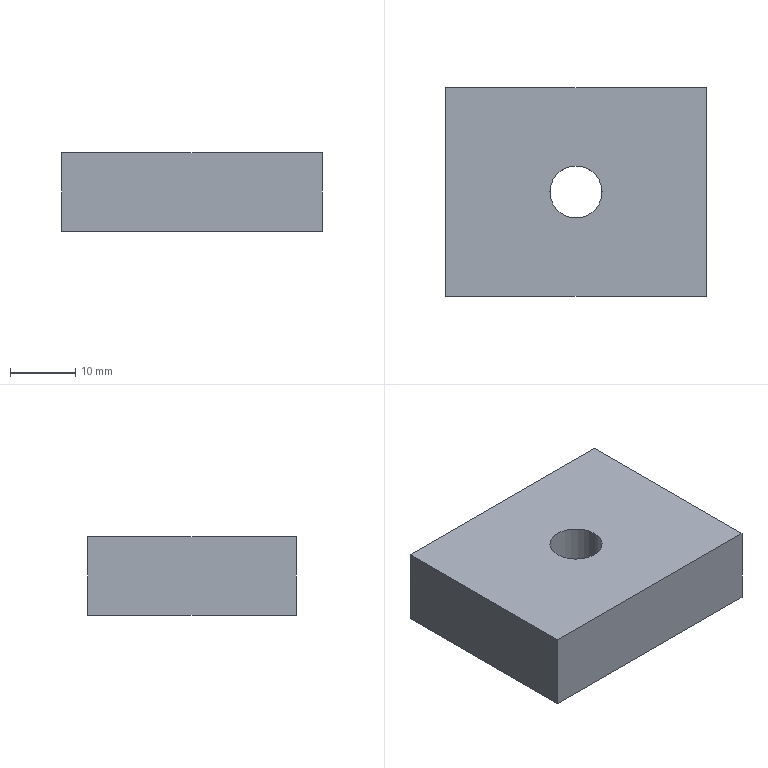Part | STEP file | [02]-4 | 1 solid | 8 faces | box 40 x 32 x 12 mm | volume 14757 mm3 | plane 6 | cylinder 2 | commonest cylinder face diameters 8 x2
STEP:
#1=CARTESIAN_POINT('',(16.,16.,0.));
#2=VERTEX_POINT('',#1);
#3=CARTESIAN_POINT('',(24.,16.,0.));
#4=VERTEX_POINT('',#3);
#5=CARTESIAN_POINT('',(20.,16.,0.));
#6=DIRECTION('',(0.,0.,1.));
#7=DIRECTION('',(1.,0.,0.));
#8=AXIS2_PLACEMENT_3D('',#5,#6,#7);
#9=CIRCLE('',#8,4.);
#10=EDGE_CURVE('',#2,#4,#9,.T.);
#11=ORIENTED_EDGE('',*,*,#10,.F.);
#12=CARTESIAN_POINT('',(16.,16.,12.));
#13=VERTEX_POINT('',#12);
#14=CARTESIAN_POINT('',(16.,16.,0.));
#15=DIRECTION('',(0.,0.,1.));
#16=VECTOR('',#15,1000.);
#17=LINE('',#14,#16);
#18=EDGE_CURVE('',#2,#13,#17,.T.);
#19=ORIENTED_EDGE('',*,*,#18,.T.);
#20=CARTESIAN_POINT('',(24.,16.,12.));
#21=VERTEX_POINT('',#20);
#22=CARTESIAN_POINT('',(20.,16.,12.));
#23=DIRECTION('',(0.,0.,-1.));
#24=DIRECTION('',(-1.,0.,0.));
#25=AXIS2_PLACEMENT_3D('',#22,#23,#24);
#26=CIRCLE('',#25,4.);
#27=EDGE_CURVE('',#21,#13,#26,.T.);
#28=ORIENTED_EDGE('',*,*,#27,.F.);
#29=CARTESIAN_POINT('',(24.,16.,0.));
#30=DIRECTION('',(0.,0.,1.));
#31=VECTOR('',#30,1000.);
#32=LINE('',#29,#31);
#33=EDGE_CURVE('',#4,#21,#32,.T.);
#34=ORIENTED_EDGE('',*,*,#33,.F.);
#35=EDGE_LOOP('',(#11,#19,#28,#34));
#36=FACE_OUTER_BOUND('',#35,.T.);
#37=CARTESIAN_POINT('',(20.,16.,0.));
#38=DIRECTION('',(0.,0.,1.));
#39=DIRECTION('',(1.,0.,0.));
#40=AXIS2_PLACEMENT_3D('',#37,#38,#39);
#41=CYLINDRICAL_SURFACE('',#40,4.);
#42=ADVANCED_FACE('',(#36),#41,.F.);
#43=CARTESIAN_POINT('',(0.,0.,0.));
#44=VERTEX_POINT('',#43);
#45=CARTESIAN_POINT('',(40.,0.,0.));
#46=VERTEX_POINT('',#45);
#47=CARTESIAN_POINT('',(20.,0.,0.));
#48=DIRECTION('',(1.,0.,0.));
#49=VECTOR('',#48,1000.);
#50=LINE('',#47,#49);
#51=EDGE_CURVE('',#44,#46,#50,.T.);
#52=ORIENTED_EDGE('',*,*,#51,.F.);
#53=CARTESIAN_POINT('',(0.,32.,0.));
#54=VERTEX_POINT('',#53);
#55=CARTESIAN_POINT('',(0.,16.,0.));
#56=DIRECTION('',(0.,-1.,0.));
#57=VECTOR('',#56,1000.);
#58=LINE('',#55,#57);
#59=EDGE_CURVE('',#54,#44,#58,.T.);
#60=ORIENTED_EDGE('',*,*,#59,.F.);
#61=CARTESIAN_POINT('',(40.,32.,0.));
#62=VERTEX_POINT('',#61);
#63=CARTESIAN_POINT('',(20.,32.,0.));
#64=DIRECTION('',(-1.,0.,0.));
#65=VECTOR('',#64,1000.);
#66=LINE('',#63,#65);
#67=EDGE_CURVE('',#62,#54,#66,.T.);
#68=ORIENTED_EDGE('',*,*,#67,.F.);
#69=CARTESIAN_POINT('',(40.,16.,0.));
#70=DIRECTION('',(0.,1.,0.));
#71=VECTOR('',#70,1000.);
#72=LINE('',#69,#71);
#73=EDGE_CURVE('',#46,#62,#72,.T.);
#74=ORIENTED_EDGE('',*,*,#73,.F.);
#75=EDGE_LOOP('',(#52,#60,#68,#74));
#76=FACE_OUTER_BOUND('',#75,.T.);
#77=CARTESIAN_POINT('',(20.,16.,0.));
#78=DIRECTION('',(0.,0.,1.));
#79=DIRECTION('',(1.,0.,0.));
#80=AXIS2_PLACEMENT_3D('',#77,#78,#79);
#81=CIRCLE('',#80,4.);
#82=EDGE_CURVE('',#4,#2,#81,.T.);
#83=ORIENTED_EDGE('',*,*,#82,.T.);
#84=ORIENTED_EDGE('',*,*,#10,.T.);
#85=EDGE_LOOP('',(#83,#84));
#86=FACE_BOUND('',#85,.T.);
#87=CARTESIAN_POINT('',(20.,16.,0.));
#88=DIRECTION('',(0.,0.,-1.));
#89=DIRECTION('',(-1.,0.,0.));
#90=AXIS2_PLACEMENT_3D('',#87,#88,#89);
#91=PLANE('',#90);
#92=ADVANCED_FACE('',(#76,#86),#91,.T.);
#93=CARTESIAN_POINT('',(0.,0.,12.));
#94=VERTEX_POINT('',#93);
#95=CARTESIAN_POINT('',(0.,0.,12.));
#96=DIRECTION('',(0.,0.,-1.));
#97=VECTOR('',#96,1000.);
#98=LINE('',#95,#97);
#99=EDGE_CURVE('',#94,#44,#98,.T.);
#100=ORIENTED_EDGE('',*,*,#99,.T.);
#101=ORIENTED_EDGE('',*,*,#51,.T.);
#102=CARTESIAN_POINT('',(40.,0.,12.));
#103=VERTEX_POINT('',#102);
#104=CARTESIAN_POINT('',(40.,0.,12.));
#105=DIRECTION('',(0.,0.,-1.));
#106=VECTOR('',#105,1000.);
#107=LINE('',#104,#106);
#108=EDGE_CURVE('',#103,#46,#107,.T.);
#109=ORIENTED_EDGE('',*,*,#108,.F.);
#110=CARTESIAN_POINT('',(20.,0.,12.));
#111=DIRECTION('',(-1.,0.,0.));
#112=VECTOR('',#111,1000.);
#113=LINE('',#110,#112);
#114=EDGE_CURVE('',#103,#94,#113,.T.);
#115=ORIENTED_EDGE('',*,*,#114,.T.);
#116=EDGE_LOOP('',(#100,#101,#109,#115));
#117=FACE_OUTER_BOUND('',#116,.T.);
#118=CARTESIAN_POINT('',(20.,0.,12.));
#119=DIRECTION('',(0.,-1.,0.));
#120=DIRECTION('',(0.,0.,1.));
#121=AXIS2_PLACEMENT_3D('',#118,#119,#120);
#122=PLANE('',#121);
#123=ADVANCED_FACE('',(#117),#122,.T.);
#124=ORIENTED_EDGE('',*,*,#108,.T.);
#125=ORIENTED_EDGE('',*,*,#73,.T.);
#126=CARTESIAN_POINT('',(40.,32.,12.));
#127=VERTEX_POINT('',#126);
#128=CARTESIAN_POINT('',(40.,32.,12.));
#129=DIRECTION('',(0.,0.,-1.));
#130=VECTOR('',#129,1000.);
#131=LINE('',#128,#130);
#132=EDGE_CURVE('',#127,#62,#131,.T.);
#133=ORIENTED_EDGE('',*,*,#132,.F.);
#134=CARTESIAN_POINT('',(40.,16.,12.));
#135=DIRECTION('',(0.,-1.,0.));
#136=VECTOR('',#135,1000.);
#137=LINE('',#134,#136);
#138=EDGE_CURVE('',#127,#103,#137,.T.);
#139=ORIENTED_EDGE('',*,*,#138,.T.);
#140=EDGE_LOOP('',(#124,#125,#133,#139));
#141=FACE_OUTER_BOUND('',#140,.T.);
#142=CARTESIAN_POINT('',(40.,16.,12.));
#143=DIRECTION('',(1.,0.,0.));
#144=DIRECTION('',(0.,0.,-1.));
#145=AXIS2_PLACEMENT_3D('',#142,#143,#144);
#146=PLANE('',#145);
#147=ADVANCED_FACE('',(#141),#146,.T.);
#148=ORIENTED_EDGE('',*,*,#132,.T.);
#149=ORIENTED_EDGE('',*,*,#67,.T.);
#150=CARTESIAN_POINT('',(0.,32.,12.));
#151=VERTEX_POINT('',#150);
#152=CARTESIAN_POINT('',(0.,32.,12.));
#153=DIRECTION('',(0.,0.,-1.));
#154=VECTOR('',#153,1000.);
#155=LINE('',#152,#154);
#156=EDGE_CURVE('',#151,#54,#155,.T.);
#157=ORIENTED_EDGE('',*,*,#156,.F.);
#158=CARTESIAN_POINT('',(20.,32.,12.));
#159=DIRECTION('',(1.,0.,0.));
#160=VECTOR('',#159,1000.);
#161=LINE('',#158,#160);
#162=EDGE_CURVE('',#151,#127,#161,.T.);
#163=ORIENTED_EDGE('',*,*,#162,.T.);
#164=EDGE_LOOP('',(#148,#149,#157,#163));
#165=FACE_OUTER_BOUND('',#164,.T.);
#166=CARTESIAN_POINT('',(20.,32.,12.));
#167=DIRECTION('',(0.,1.,0.));
#168=DIRECTION('',(0.,0.,-1.));
#169=AXIS2_PLACEMENT_3D('',#166,#167,#168);
#170=PLANE('',#169);
#171=ADVANCED_FACE('',(#165),#170,.T.);
#172=ORIENTED_EDGE('',*,*,#27,.T.);
#173=CARTESIAN_POINT('',(20.,16.,12.));
#174=DIRECTION('',(0.,0.,-1.));
#175=DIRECTION('',(-1.,0.,0.));
#176=AXIS2_PLACEMENT_3D('',#173,#174,#175);
#177=CIRCLE('',#176,4.);
#178=EDGE_CURVE('',#13,#21,#177,.T.);
#179=ORIENTED_EDGE('',*,*,#178,.T.);
#180=EDGE_LOOP('',(#172,#179));
#181=FACE_BOUND('',#180,.T.);
#182=CARTESIAN_POINT('',(0.,16.,12.));
#183=DIRECTION('',(0.,1.,0.));
#184=VECTOR('',#183,1000.);
#185=LINE('',#182,#184);
#186=EDGE_CURVE('',#94,#151,#185,.T.);
#187=ORIENTED_EDGE('',*,*,#186,.F.);
#188=ORIENTED_EDGE('',*,*,#114,.F.);
#189=ORIENTED_EDGE('',*,*,#138,.F.);
#190=ORIENTED_EDGE('',*,*,#162,.F.);
#191=EDGE_LOOP('',(#187,#188,#189,#190));
#192=FACE_OUTER_BOUND('',#191,.T.);
#193=CARTESIAN_POINT('',(20.,16.,12.));
#194=DIRECTION('',(0.,0.,1.));
#195=DIRECTION('',(1.,0.,0.));
#196=AXIS2_PLACEMENT_3D('',#193,#194,#195);
#197=PLANE('',#196);
#198=ADVANCED_FACE('',(#181,#192),#197,.T.);
#199=ORIENTED_EDGE('',*,*,#186,.T.);
#200=ORIENTED_EDGE('',*,*,#156,.T.);
#201=ORIENTED_EDGE('',*,*,#59,.T.);
#202=ORIENTED_EDGE('',*,*,#99,.F.);
#203=EDGE_LOOP('',(#199,#200,#201,#202));
#204=FACE_OUTER_BOUND('',#203,.T.);
#205=CARTESIAN_POINT('',(0.,16.,12.));
#206=DIRECTION('',(-1.,0.,0.));
#207=DIRECTION('',(0.,0.,1.));
#208=AXIS2_PLACEMENT_3D('',#205,#206,#207);
#209=PLANE('',#208);
#210=ADVANCED_FACE('',(#204),#209,.T.);
#211=ORIENTED_EDGE('',*,*,#18,.F.);
#212=ORIENTED_EDGE('',*,*,#82,.F.);
#213=ORIENTED_EDGE('',*,*,#33,.T.);
#214=ORIENTED_EDGE('',*,*,#178,.F.);
#215=EDGE_LOOP('',(#211,#212,#213,#214));
#216=FACE_OUTER_BOUND('',#215,.T.);
#217=CARTESIAN_POINT('',(20.,16.,0.));
#218=DIRECTION('',(0.,0.,1.));
#219=DIRECTION('',(1.,0.,0.));
#220=AXIS2_PLACEMENT_3D('',#217,#218,#219);
#221=CYLINDRICAL_SURFACE('',#220,4.);
#222=ADVANCED_FACE('',(#216),#221,.F.);
#223=CLOSED_SHELL('',(#42,#92,#123,#147,#171,#198,#210,#222));
#224=MANIFOLD_SOLID_BREP('',#223);
#225=CARTESIAN_POINT('',(0.,0.,0.));
#226=DIRECTION('',(0.,0.,1.));
#227=DIRECTION('',(1.,0.,0.));
#228=AXIS2_PLACEMENT_3D('',#225,#226,#227);
#229=(LENGTH_UNIT()NAMED_UNIT(*)SI_UNIT(.MILLI.,.METRE.));
#230=UNCERTAINTY_MEASURE_WITH_UNIT(LENGTH_MEASURE(0.00001),#229,'','');
#231=(NAMED_UNIT(*)PLANE_ANGLE_UNIT()SI_UNIT($,.RADIAN.));
#232=(NAMED_UNIT(*)SI_UNIT($,.STERADIAN.)SOLID_ANGLE_UNIT());
#233=(GEOMETRIC_REPRESENTATION_CONTEXT(3)GLOBAL_UNCERTAINTY_ASSIGNED_CONTEXT((#230))GLOBAL_UNIT_ASSIGNED_CONTEXT((#229,#231,#232))REPRESENTATION_CONTEXT('',''));
#234=ADVANCED_BREP_SHAPE_REPRESENTATION('',(#224,#228),#233);